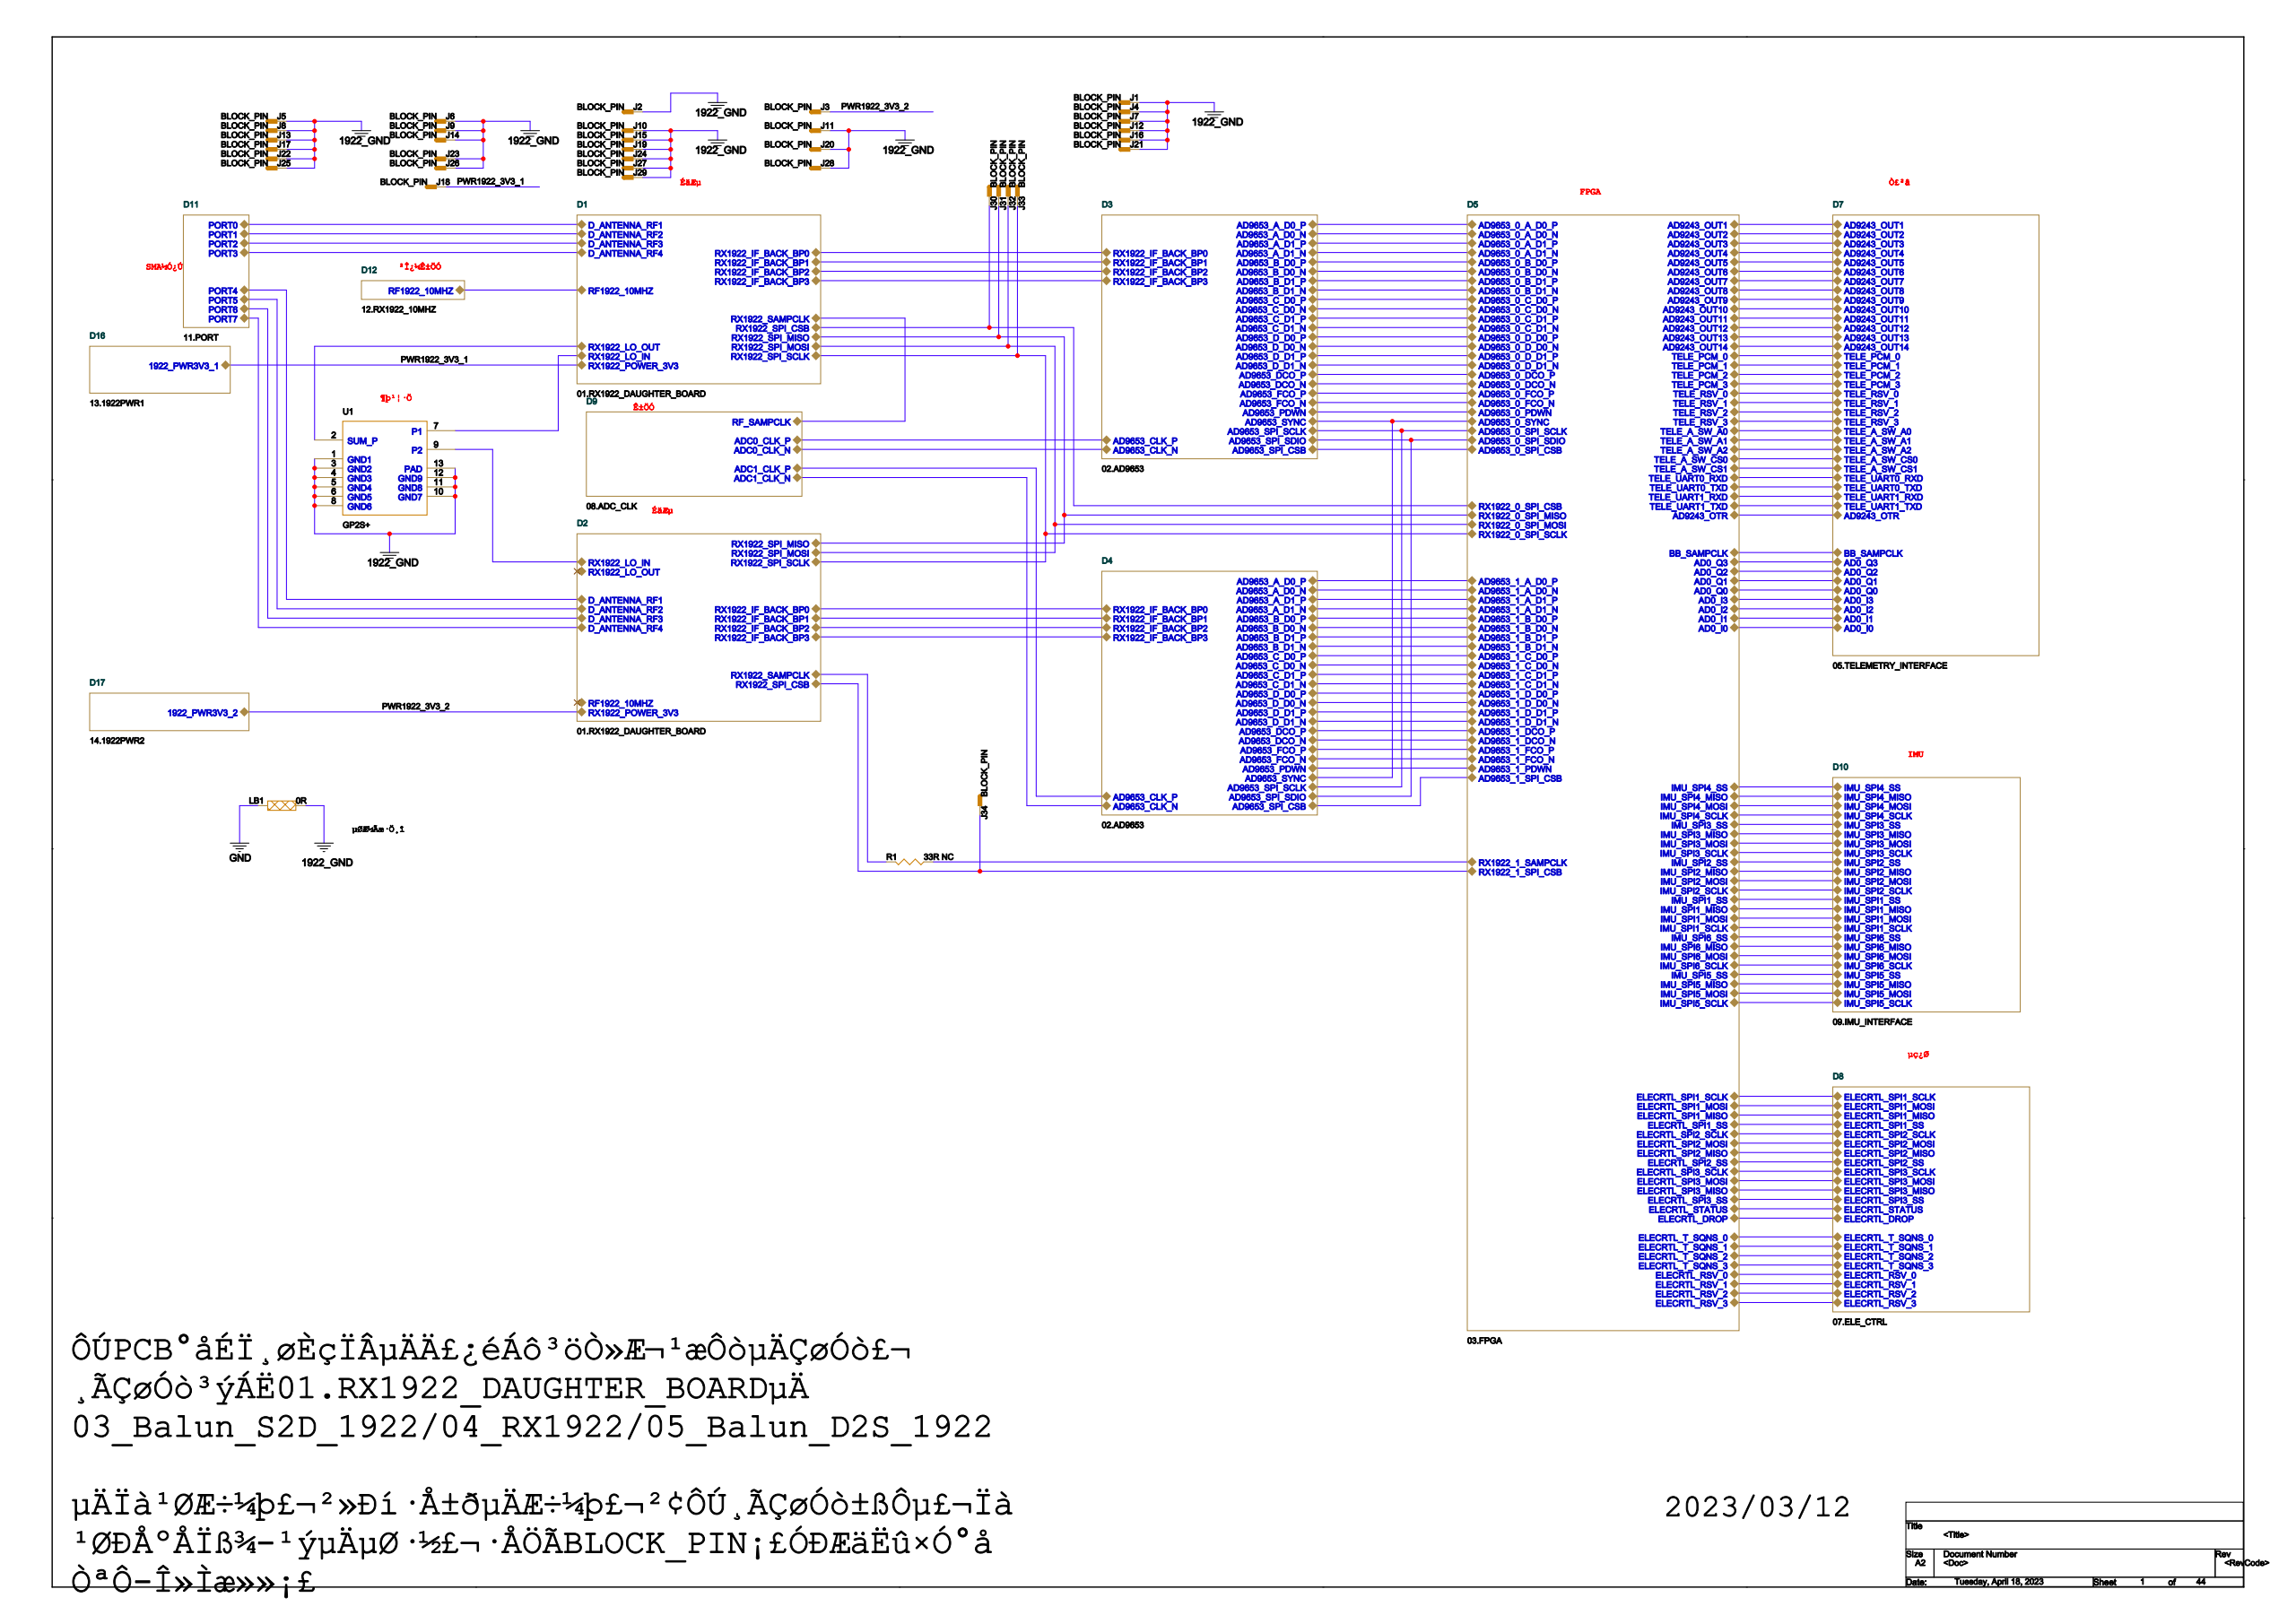Circuit board | Cadence Allegro | 1034 parts | 912 nets | one sheet of the schematic
Parts on this sheet (reference | value | footprint):
J1 | BLOCK_PIN | B_PIN_SMD
J2 | BLOCK_PIN | B_PIN_SMD
J3 | BLOCK_PIN | B_PIN_SMD
J4 | BLOCK_PIN | B_PIN_SMD
J5 | BLOCK_PIN | B_PIN_SMD
J6 | BLOCK_PIN | B_PIN_SMD
J7 | BLOCK_PIN | B_PIN_SMD
J8 | BLOCK_PIN | B_PIN_SMD
J9 | BLOCK_PIN | B_PIN_SMD
J10 | BLOCK_PIN | B_PIN_SMD
J11 | BLOCK_PIN | B_PIN_SMD
J12 | BLOCK_PIN | B_PIN_SMD
J13 | BLOCK_PIN | B_PIN_SMD
J14 | BLOCK_PIN | B_PIN_SMD
J15 | BLOCK_PIN | B_PIN_SMD
J16 | BLOCK_PIN | B_PIN_SMD
J17 | BLOCK_PIN | B_PIN_SMD
J18 | BLOCK_PIN | B_PIN_SMD
J19 | BLOCK_PIN | B_PIN_SMD
J20 | BLOCK_PIN | B_PIN_SMD
J21 | BLOCK_PIN | B_PIN_SMD
J22 | BLOCK_PIN | B_PIN_SMD
J23 | BLOCK_PIN | B_PIN_SMD
J24 | BLOCK_PIN | B_PIN_SMD
J25 | BLOCK_PIN | B_PIN_SMD
J26 | BLOCK_PIN | B_PIN_SMD
J27 | BLOCK_PIN | B_PIN_SMD
J28 | BLOCK_PIN | B_PIN_SMD
J29 | BLOCK_PIN | B_PIN_SMD
J30 | BLOCK_PIN | B_PIN_SMD
J31 | BLOCK_PIN | B_PIN_SMD
J32 | BLOCK_PIN | B_PIN_SMD
J33 | BLOCK_PIN | B_PIN_SMD
J34 | BLOCK_PIN | B_PIN_SMD
LB1 | 0R | LB0805
P1 | TSW-120-07-G-D | TSW_2MM54_DR
U1 | GP2S+ | GP2S_PS
Nets of these parts (net: part-pin ...):
GND: LB1-1 P1-1 P1-2 P1-3 P1-4 P1-9 P1-10
N188146: J33-1
N188086: J34-1
1922_GND: J1-1 J2-1 J4-1 J5-1 J6-1 J7-1 J8-1 J9-1 J10-1 J11-1 J12-1 J13-1 J14-1 J15-1 J16-1 J17-1 J19-1 J20-1 J21-1 J22-1 J23-1 J24-1 J25-1 J26-1 J27-1 J28-1 J29-1 LB1-2 U1-1 U1-3 U1-4 U1-5 U1-6 U1-8 U1-10 U1-11 U1-12 U1-13
PWR1922_3V3_2: J3-1
PWR1922_3V3_1: J18-1
N188122: J30-1
N188134: J31-1
N251303: J32-1
N246478: U1-7
N246591: U1-9
N244746: U1-2